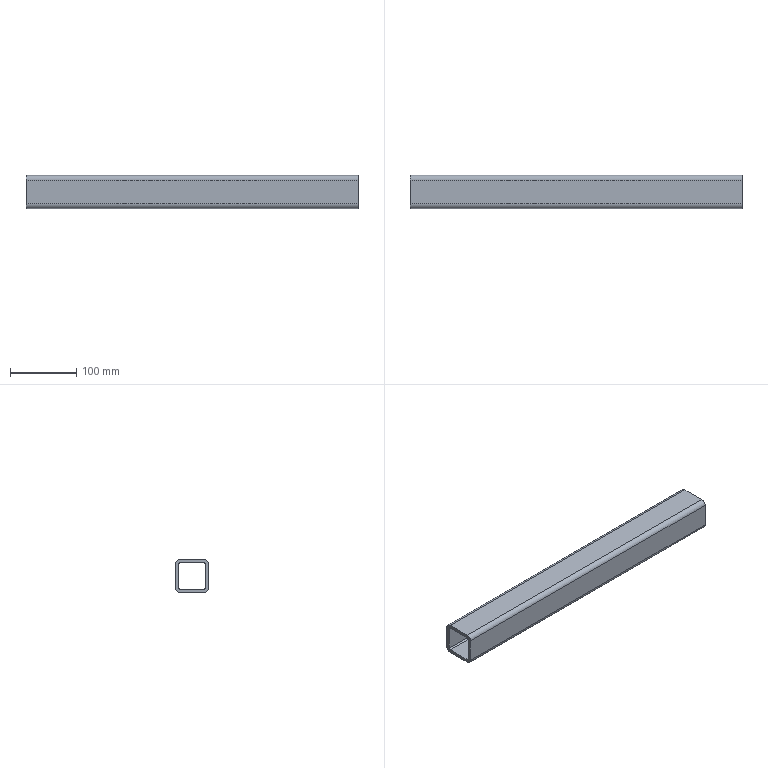Part | NX | 1 solid | 18 faces | box 500 x 50 x 50 mm | volume 430686 mm3 | plane 10 | cylinder 8 | commonest cylinder face diameters 4 x4 14 x4
STEP:
#1=CARTESIAN_POINT('',(-850.,18.,290.));
#2=VERTEX_POINT('',#1);
#3=CARTESIAN_POINT('',(-350.,18.,290.));
#4=VERTEX_POINT('',#3);
#5=CARTESIAN_POINT('',(-875.,18.,290.));
#6=DIRECTION('',(1.,0.,0.));
#7=VECTOR('',#6,1000.);
#8=LINE('',#5,#7);
#9=EDGE_CURVE('',#2,#4,#8,.T.);
#10=ORIENTED_EDGE('',*,*,#9,.F.);
#11=CARTESIAN_POINT('',(-850.,-18.,290.));
#12=VERTEX_POINT('',#11);
#13=CARTESIAN_POINT('',(-850.,-18.,290.));
#14=DIRECTION('',(0.,-1.,0.));
#15=VECTOR('',#14,1000.);
#16=LINE('',#13,#15);
#17=EDGE_CURVE('',#2,#12,#16,.T.);
#18=ORIENTED_EDGE('',*,*,#17,.T.);
#19=CARTESIAN_POINT('',(-350.,-18.,290.));
#20=VERTEX_POINT('',#19);
#21=CARTESIAN_POINT('',(-875.,-18.,290.));
#22=DIRECTION('',(1.,0.,0.));
#23=VECTOR('',#22,1000.);
#24=LINE('',#21,#23);
#25=EDGE_CURVE('',#12,#20,#24,.T.);
#26=ORIENTED_EDGE('',*,*,#25,.T.);
#27=CARTESIAN_POINT('',(-350.,-18.,290.));
#28=DIRECTION('',(0.,1.,0.));
#29=VECTOR('',#28,1000.);
#30=LINE('',#27,#29);
#31=EDGE_CURVE('',#20,#4,#30,.T.);
#32=ORIENTED_EDGE('',*,*,#31,.T.);
#33=EDGE_LOOP('',(#10,#18,#26,#32));
#34=FACE_BOUND('',#33,.T.);
#35=CARTESIAN_POINT('',(-875.,-18.,290.));
#36=DIRECTION('',(0.,0.,1.));
#37=DIRECTION('',(1.,0.,0.));
#38=AXIS2_PLACEMENT_3D('',#35,#36,#37);
#39=PLANE('',#38);
#40=ADVANCED_FACE('',(#34),#39,.T.);
#41=ORIENTED_EDGE('',*,*,#25,.F.);
#42=CARTESIAN_POINT('',(-850.,-20.,292.));
#43=VERTEX_POINT('',#42);
#44=CARTESIAN_POINT('',(-850.,-18.,292.));
#45=DIRECTION('',(-1.,0.,0.));
#46=DIRECTION('',(0.,0.,1.));
#47=AXIS2_PLACEMENT_3D('',#44,#45,#46);
#48=CIRCLE('',#47,2.);
#49=EDGE_CURVE('',#12,#43,#48,.T.);
#50=ORIENTED_EDGE('',*,*,#49,.T.);
#51=CARTESIAN_POINT('',(-350.,-20.,292.));
#52=VERTEX_POINT('',#51);
#53=CARTESIAN_POINT('',(-875.,-20.,292.));
#54=DIRECTION('',(1.,0.,0.));
#55=VECTOR('',#54,1000.);
#56=LINE('',#53,#55);
#57=EDGE_CURVE('',#43,#52,#56,.T.);
#58=ORIENTED_EDGE('',*,*,#57,.T.);
#59=CARTESIAN_POINT('',(-350.,-18.,292.));
#60=DIRECTION('',(1.,0.,0.));
#61=DIRECTION('',(0.,1.,0.));
#62=AXIS2_PLACEMENT_3D('',#59,#60,#61);
#63=CIRCLE('',#62,2.);
#64=EDGE_CURVE('',#52,#20,#63,.T.);
#65=ORIENTED_EDGE('',*,*,#64,.T.);
#66=EDGE_LOOP('',(#41,#50,#58,#65));
#67=FACE_BOUND('',#66,.T.);
#68=CARTESIAN_POINT('',(-875.,-18.,292.));
#69=DIRECTION('',(1.,0.,0.));
#70=DIRECTION('',(0.,0.,-1.));
#71=AXIS2_PLACEMENT_3D('',#68,#69,#70);
#72=CYLINDRICAL_SURFACE('',#71,2.);
#73=ADVANCED_FACE('',(#67),#72,.F.);
#74=ORIENTED_EDGE('',*,*,#57,.F.);
#75=CARTESIAN_POINT('',(-850.,-20.,328.));
#76=VERTEX_POINT('',#75);
#77=CARTESIAN_POINT('',(-850.,-20.,292.));
#78=DIRECTION('',(0.,0.,1.));
#79=VECTOR('',#78,1000.);
#80=LINE('',#77,#79);
#81=EDGE_CURVE('',#43,#76,#80,.T.);
#82=ORIENTED_EDGE('',*,*,#81,.T.);
#83=CARTESIAN_POINT('',(-350.,-20.,328.));
#84=VERTEX_POINT('',#83);
#85=CARTESIAN_POINT('',(-875.,-20.,328.));
#86=DIRECTION('',(1.,0.,0.));
#87=VECTOR('',#86,1000.);
#88=LINE('',#85,#87);
#89=EDGE_CURVE('',#76,#84,#88,.T.);
#90=ORIENTED_EDGE('',*,*,#89,.T.);
#91=CARTESIAN_POINT('',(-350.,-20.,292.));
#92=DIRECTION('',(0.,0.,-1.));
#93=VECTOR('',#92,1000.);
#94=LINE('',#91,#93);
#95=EDGE_CURVE('',#84,#52,#94,.T.);
#96=ORIENTED_EDGE('',*,*,#95,.T.);
#97=EDGE_LOOP('',(#74,#82,#90,#96));
#98=FACE_BOUND('',#97,.T.);
#99=CARTESIAN_POINT('',(-875.,-20.,292.));
#100=DIRECTION('',(0.,1.,0.));
#101=DIRECTION('',(0.,0.,1.));
#102=AXIS2_PLACEMENT_3D('',#99,#100,#101);
#103=PLANE('',#102);
#104=ADVANCED_FACE('',(#98),#103,.T.);
#105=ORIENTED_EDGE('',*,*,#89,.F.);
#106=CARTESIAN_POINT('',(-850.,-18.,330.));
#107=VERTEX_POINT('',#106);
#108=CARTESIAN_POINT('',(-850.,-18.,328.));
#109=DIRECTION('',(-1.,0.,0.));
#110=DIRECTION('',(0.,0.,1.));
#111=AXIS2_PLACEMENT_3D('',#108,#109,#110);
#112=CIRCLE('',#111,2.);
#113=EDGE_CURVE('',#76,#107,#112,.T.);
#114=ORIENTED_EDGE('',*,*,#113,.T.);
#115=CARTESIAN_POINT('',(-350.,-18.,330.));
#116=VERTEX_POINT('',#115);
#117=CARTESIAN_POINT('',(-875.,-18.,330.));
#118=DIRECTION('',(1.,0.,0.));
#119=VECTOR('',#118,1000.);
#120=LINE('',#117,#119);
#121=EDGE_CURVE('',#107,#116,#120,.T.);
#122=ORIENTED_EDGE('',*,*,#121,.T.);
#123=CARTESIAN_POINT('',(-350.,-18.,328.));
#124=DIRECTION('',(1.,0.,0.));
#125=DIRECTION('',(0.,1.,0.));
#126=AXIS2_PLACEMENT_3D('',#123,#124,#125);
#127=CIRCLE('',#126,2.);
#128=EDGE_CURVE('',#116,#84,#127,.T.);
#129=ORIENTED_EDGE('',*,*,#128,.T.);
#130=EDGE_LOOP('',(#105,#114,#122,#129));
#131=FACE_BOUND('',#130,.T.);
#132=CARTESIAN_POINT('',(-875.,-18.,328.));
#133=DIRECTION('',(1.,0.,0.));
#134=DIRECTION('',(0.,0.,-1.));
#135=AXIS2_PLACEMENT_3D('',#132,#133,#134);
#136=CYLINDRICAL_SURFACE('',#135,2.);
#137=ADVANCED_FACE('',(#131),#136,.F.);
#138=ORIENTED_EDGE('',*,*,#121,.F.);
#139=CARTESIAN_POINT('',(-850.,18.,330.));
#140=VERTEX_POINT('',#139);
#141=CARTESIAN_POINT('',(-850.,18.,330.));
#142=DIRECTION('',(0.,1.,0.));
#143=VECTOR('',#142,1000.);
#144=LINE('',#141,#143);
#145=EDGE_CURVE('',#107,#140,#144,.T.);
#146=ORIENTED_EDGE('',*,*,#145,.T.);
#147=CARTESIAN_POINT('',(-350.,18.,330.));
#148=VERTEX_POINT('',#147);
#149=CARTESIAN_POINT('',(-875.,18.,330.));
#150=DIRECTION('',(1.,0.,0.));
#151=VECTOR('',#150,1000.);
#152=LINE('',#149,#151);
#153=EDGE_CURVE('',#140,#148,#152,.T.);
#154=ORIENTED_EDGE('',*,*,#153,.T.);
#155=CARTESIAN_POINT('',(-350.,18.,330.));
#156=DIRECTION('',(0.,-1.,0.));
#157=VECTOR('',#156,1000.);
#158=LINE('',#155,#157);
#159=EDGE_CURVE('',#148,#116,#158,.T.);
#160=ORIENTED_EDGE('',*,*,#159,.T.);
#161=EDGE_LOOP('',(#138,#146,#154,#160));
#162=FACE_BOUND('',#161,.T.);
#163=CARTESIAN_POINT('',(-875.,18.,330.));
#164=DIRECTION('',(0.,0.,-1.));
#165=DIRECTION('',(-1.,0.,0.));
#166=AXIS2_PLACEMENT_3D('',#163,#164,#165);
#167=PLANE('',#166);
#168=ADVANCED_FACE('',(#162),#167,.T.);
#169=ORIENTED_EDGE('',*,*,#153,.F.);
#170=CARTESIAN_POINT('',(-850.,20.,328.));
#171=VERTEX_POINT('',#170);
#172=CARTESIAN_POINT('',(-850.,18.,328.));
#173=DIRECTION('',(-1.,0.,0.));
#174=DIRECTION('',(0.,0.,1.));
#175=AXIS2_PLACEMENT_3D('',#172,#173,#174);
#176=CIRCLE('',#175,2.);
#177=EDGE_CURVE('',#140,#171,#176,.T.);
#178=ORIENTED_EDGE('',*,*,#177,.T.);
#179=CARTESIAN_POINT('',(-350.,20.,328.));
#180=VERTEX_POINT('',#179);
#181=CARTESIAN_POINT('',(-875.,20.,328.));
#182=DIRECTION('',(1.,0.,0.));
#183=VECTOR('',#182,1000.);
#184=LINE('',#181,#183);
#185=EDGE_CURVE('',#171,#180,#184,.T.);
#186=ORIENTED_EDGE('',*,*,#185,.T.);
#187=CARTESIAN_POINT('',(-350.,18.,328.));
#188=DIRECTION('',(1.,0.,0.));
#189=DIRECTION('',(0.,1.,0.));
#190=AXIS2_PLACEMENT_3D('',#187,#188,#189);
#191=CIRCLE('',#190,2.);
#192=EDGE_CURVE('',#180,#148,#191,.T.);
#193=ORIENTED_EDGE('',*,*,#192,.T.);
#194=EDGE_LOOP('',(#169,#178,#186,#193));
#195=FACE_BOUND('',#194,.T.);
#196=CARTESIAN_POINT('',(-875.,18.,328.));
#197=DIRECTION('',(1.,0.,0.));
#198=DIRECTION('',(0.,0.,-1.));
#199=AXIS2_PLACEMENT_3D('',#196,#197,#198);
#200=CYLINDRICAL_SURFACE('',#199,2.);
#201=ADVANCED_FACE('',(#195),#200,.F.);
#202=ORIENTED_EDGE('',*,*,#185,.F.);
#203=CARTESIAN_POINT('',(-850.,20.,292.));
#204=VERTEX_POINT('',#203);
#205=CARTESIAN_POINT('',(-850.,20.,328.));
#206=DIRECTION('',(0.,0.,-1.));
#207=VECTOR('',#206,1000.);
#208=LINE('',#205,#207);
#209=EDGE_CURVE('',#171,#204,#208,.T.);
#210=ORIENTED_EDGE('',*,*,#209,.T.);
#211=CARTESIAN_POINT('',(-350.,20.,292.));
#212=VERTEX_POINT('',#211);
#213=CARTESIAN_POINT('',(-875.,20.,292.));
#214=DIRECTION('',(1.,0.,0.));
#215=VECTOR('',#214,1000.);
#216=LINE('',#213,#215);
#217=EDGE_CURVE('',#204,#212,#216,.T.);
#218=ORIENTED_EDGE('',*,*,#217,.T.);
#219=CARTESIAN_POINT('',(-350.,20.,328.));
#220=DIRECTION('',(0.,0.,1.));
#221=VECTOR('',#220,1000.);
#222=LINE('',#219,#221);
#223=EDGE_CURVE('',#212,#180,#222,.T.);
#224=ORIENTED_EDGE('',*,*,#223,.T.);
#225=EDGE_LOOP('',(#202,#210,#218,#224));
#226=FACE_BOUND('',#225,.T.);
#227=CARTESIAN_POINT('',(-875.,20.,328.));
#228=DIRECTION('',(0.,-1.,0.));
#229=DIRECTION('',(0.,0.,-1.));
#230=AXIS2_PLACEMENT_3D('',#227,#228,#229);
#231=PLANE('',#230);
#232=ADVANCED_FACE('',(#226),#231,.T.);
#233=ORIENTED_EDGE('',*,*,#217,.F.);
#234=CARTESIAN_POINT('',(-850.,18.,292.));
#235=DIRECTION('',(-1.,0.,0.));
#236=DIRECTION('',(0.,0.,1.));
#237=AXIS2_PLACEMENT_3D('',#234,#235,#236);
#238=CIRCLE('',#237,2.);
#239=EDGE_CURVE('',#204,#2,#238,.T.);
#240=ORIENTED_EDGE('',*,*,#239,.T.);
#241=ORIENTED_EDGE('',*,*,#9,.T.);
#242=CARTESIAN_POINT('',(-350.,18.,292.));
#243=DIRECTION('',(1.,0.,0.));
#244=DIRECTION('',(0.,1.,0.));
#245=AXIS2_PLACEMENT_3D('',#242,#243,#244);
#246=CIRCLE('',#245,2.);
#247=EDGE_CURVE('',#4,#212,#246,.T.);
#248=ORIENTED_EDGE('',*,*,#247,.T.);
#249=EDGE_LOOP('',(#233,#240,#241,#248));
#250=FACE_BOUND('',#249,.T.);
#251=CARTESIAN_POINT('',(-875.,18.,292.));
#252=DIRECTION('',(1.,0.,0.));
#253=DIRECTION('',(0.,0.,-1.));
#254=AXIS2_PLACEMENT_3D('',#251,#252,#253);
#255=CYLINDRICAL_SURFACE('',#254,2.);
#256=ADVANCED_FACE('',(#250),#255,.F.);
#257=CARTESIAN_POINT('',(-850.,-18.,335.));
#258=VERTEX_POINT('',#257);
#259=CARTESIAN_POINT('',(-850.,18.,335.));
#260=VERTEX_POINT('',#259);
#261=CARTESIAN_POINT('',(-850.,0.,335.));
#262=DIRECTION('',(0.,1.,0.));
#263=VECTOR('',#262,1000.);
#264=LINE('',#261,#263);
#265=EDGE_CURVE('',#258,#260,#264,.T.);
#266=ORIENTED_EDGE('',*,*,#265,.F.);
#267=CARTESIAN_POINT('',(-350.,-18.,335.));
#268=VERTEX_POINT('',#267);
#269=CARTESIAN_POINT('',(-875.,-18.,335.));
#270=DIRECTION('',(1.,0.,0.));
#271=VECTOR('',#270,1000.);
#272=LINE('',#269,#271);
#273=EDGE_CURVE('',#258,#268,#272,.T.);
#274=ORIENTED_EDGE('',*,*,#273,.T.);
#275=CARTESIAN_POINT('',(-350.,18.,335.));
#276=VERTEX_POINT('',#275);
#277=CARTESIAN_POINT('',(-350.,18.,335.));
#278=DIRECTION('',(0.,-1.,0.));
#279=VECTOR('',#278,1000.);
#280=LINE('',#277,#279);
#281=EDGE_CURVE('',#276,#268,#280,.T.);
#282=ORIENTED_EDGE('',*,*,#281,.F.);
#283=CARTESIAN_POINT('',(-875.,18.,335.));
#284=DIRECTION('',(1.,0.,0.));
#285=VECTOR('',#284,1000.);
#286=LINE('',#283,#285);
#287=EDGE_CURVE('',#260,#276,#286,.T.);
#288=ORIENTED_EDGE('',*,*,#287,.F.);
#289=EDGE_LOOP('',(#266,#274,#282,#288));
#290=FACE_BOUND('',#289,.T.);
#291=CARTESIAN_POINT('',(-875.,18.,335.));
#292=DIRECTION('',(0.,0.,-1.));
#293=DIRECTION('',(-1.,0.,0.));
#294=AXIS2_PLACEMENT_3D('',#291,#292,#293);
#295=PLANE('',#294);
#296=ADVANCED_FACE('',(#290),#295,.F.);
#297=CARTESIAN_POINT('',(-850.,-25.,328.));
#298=VERTEX_POINT('',#297);
#299=CARTESIAN_POINT('',(-850.,-18.,328.));
#300=DIRECTION('',(-1.,0.,0.));
#301=DIRECTION('',(0.,0.,1.));
#302=AXIS2_PLACEMENT_3D('',#299,#300,#301);
#303=CIRCLE('',#302,7.);
#304=EDGE_CURVE('',#298,#258,#303,.T.);
#305=ORIENTED_EDGE('',*,*,#304,.F.);
#306=CARTESIAN_POINT('',(-350.,-25.,328.));
#307=VERTEX_POINT('',#306);
#308=CARTESIAN_POINT('',(-875.,-25.,328.));
#309=DIRECTION('',(1.,0.,0.));
#310=VECTOR('',#309,1000.);
#311=LINE('',#308,#310);
#312=EDGE_CURVE('',#298,#307,#311,.T.);
#313=ORIENTED_EDGE('',*,*,#312,.T.);
#314=CARTESIAN_POINT('',(-350.,-18.,328.));
#315=DIRECTION('',(1.,0.,0.));
#316=DIRECTION('',(0.,1.,0.));
#317=AXIS2_PLACEMENT_3D('',#314,#315,#316);
#318=CIRCLE('',#317,7.);
#319=EDGE_CURVE('',#268,#307,#318,.T.);
#320=ORIENTED_EDGE('',*,*,#319,.F.);
#321=ORIENTED_EDGE('',*,*,#273,.F.);
#322=EDGE_LOOP('',(#305,#313,#320,#321));
#323=FACE_BOUND('',#322,.T.);
#324=CARTESIAN_POINT('',(-875.,-18.,328.));
#325=DIRECTION('',(1.,0.,0.));
#326=DIRECTION('',(0.,0.,-1.));
#327=AXIS2_PLACEMENT_3D('',#324,#325,#326);
#328=CYLINDRICAL_SURFACE('',#327,7.);
#329=ADVANCED_FACE('',(#323),#328,.T.);
#330=CARTESIAN_POINT('',(-850.,-25.,292.));
#331=VERTEX_POINT('',#330);
#332=CARTESIAN_POINT('',(-850.,-25.,292.));
#333=DIRECTION('',(0.,0.,1.));
#334=VECTOR('',#333,1000.);
#335=LINE('',#332,#334);
#336=EDGE_CURVE('',#331,#298,#335,.T.);
#337=ORIENTED_EDGE('',*,*,#336,.F.);
#338=CARTESIAN_POINT('',(-350.,-25.,292.));
#339=VERTEX_POINT('',#338);
#340=CARTESIAN_POINT('',(-875.,-25.,292.));
#341=DIRECTION('',(1.,0.,0.));
#342=VECTOR('',#341,1000.);
#343=LINE('',#340,#342);
#344=EDGE_CURVE('',#331,#339,#343,.T.);
#345=ORIENTED_EDGE('',*,*,#344,.T.);
#346=CARTESIAN_POINT('',(-350.,-25.,575.));
#347=DIRECTION('',(0.,0.,-1.));
#348=VECTOR('',#347,1000.);
#349=LINE('',#346,#348);
#350=EDGE_CURVE('',#307,#339,#349,.T.);
#351=ORIENTED_EDGE('',*,*,#350,.F.);
#352=ORIENTED_EDGE('',*,*,#312,.F.);
#353=EDGE_LOOP('',(#337,#345,#351,#352));
#354=FACE_BOUND('',#353,.T.);
#355=CARTESIAN_POINT('',(-875.,-25.,292.));
#356=DIRECTION('',(0.,1.,0.));
#357=DIRECTION('',(0.,0.,1.));
#358=AXIS2_PLACEMENT_3D('',#355,#356,#357);
#359=PLANE('',#358);
#360=ADVANCED_FACE('',(#354),#359,.F.);
#361=CARTESIAN_POINT('',(-850.,-18.,285.));
#362=VERTEX_POINT('',#361);
#363=CARTESIAN_POINT('',(-850.,-18.,292.));
#364=DIRECTION('',(-1.,0.,0.));
#365=DIRECTION('',(0.,0.,1.));
#366=AXIS2_PLACEMENT_3D('',#363,#364,#365);
#367=CIRCLE('',#366,7.);
#368=EDGE_CURVE('',#362,#331,#367,.T.);
#369=ORIENTED_EDGE('',*,*,#368,.F.);
#370=CARTESIAN_POINT('',(-350.,-18.,285.));
#371=VERTEX_POINT('',#370);
#372=CARTESIAN_POINT('',(-875.,-18.,285.));
#373=DIRECTION('',(1.,0.,0.));
#374=VECTOR('',#373,1000.);
#375=LINE('',#372,#374);
#376=EDGE_CURVE('',#362,#371,#375,.T.);
#377=ORIENTED_EDGE('',*,*,#376,.T.);
#378=CARTESIAN_POINT('',(-350.,-18.,292.));
#379=DIRECTION('',(1.,0.,0.));
#380=DIRECTION('',(0.,1.,0.));
#381=AXIS2_PLACEMENT_3D('',#378,#379,#380);
#382=CIRCLE('',#381,7.);
#383=EDGE_CURVE('',#339,#371,#382,.T.);
#384=ORIENTED_EDGE('',*,*,#383,.F.);
#385=ORIENTED_EDGE('',*,*,#344,.F.);
#386=EDGE_LOOP('',(#369,#377,#384,#385));
#387=FACE_BOUND('',#386,.T.);
#388=CARTESIAN_POINT('',(-875.,-18.,292.));
#389=DIRECTION('',(1.,0.,0.));
#390=DIRECTION('',(0.,0.,-1.));
#391=AXIS2_PLACEMENT_3D('',#388,#389,#390);
#392=CYLINDRICAL_SURFACE('',#391,7.);
#393=ADVANCED_FACE('',(#387),#392,.T.);
#394=CARTESIAN_POINT('',(-850.,18.,285.));
#395=VERTEX_POINT('',#394);
#396=CARTESIAN_POINT('',(-850.,0.,285.));
#397=DIRECTION('',(0.,1.,0.));
#398=VECTOR('',#397,1000.);
#399=LINE('',#396,#398);
#400=EDGE_CURVE('',#362,#395,#399,.T.);
#401=ORIENTED_EDGE('',*,*,#400,.T.);
#402=CARTESIAN_POINT('',(-350.,18.,285.));
#403=VERTEX_POINT('',#402);
#404=CARTESIAN_POINT('',(-875.,18.,285.));
#405=DIRECTION('',(1.,0.,0.));
#406=VECTOR('',#405,1000.);
#407=LINE('',#404,#406);
#408=EDGE_CURVE('',#395,#403,#407,.T.);
#409=ORIENTED_EDGE('',*,*,#408,.T.);
#410=CARTESIAN_POINT('',(-350.,-18.,285.));
#411=DIRECTION('',(0.,1.,0.));
#412=VECTOR('',#411,1000.);
#413=LINE('',#410,#412);
#414=EDGE_CURVE('',#371,#403,#413,.T.);
#415=ORIENTED_EDGE('',*,*,#414,.F.);
#416=ORIENTED_EDGE('',*,*,#376,.F.);
#417=EDGE_LOOP('',(#401,#409,#415,#416));
#418=FACE_BOUND('',#417,.T.);
#419=CARTESIAN_POINT('',(-875.,-18.,285.));
#420=DIRECTION('',(0.,0.,1.));
#421=DIRECTION('',(1.,0.,0.));
#422=AXIS2_PLACEMENT_3D('',#419,#420,#421);
#423=PLANE('',#422);
#424=ADVANCED_FACE('',(#418),#423,.F.);
#425=CARTESIAN_POINT('',(-850.,25.,292.));
#426=VERTEX_POINT('',#425);
#427=CARTESIAN_POINT('',(-850.,18.,292.));
#428=DIRECTION('',(-1.,0.,0.));
#429=DIRECTION('',(0.,0.,1.));
#430=AXIS2_PLACEMENT_3D('',#427,#428,#429);
#431=CIRCLE('',#430,7.);
#432=EDGE_CURVE('',#426,#395,#431,.T.);
#433=ORIENTED_EDGE('',*,*,#432,.F.);
#434=CARTESIAN_POINT('',(-350.,25.,292.));
#435=VERTEX_POINT('',#434);
#436=CARTESIAN_POINT('',(-875.,25.,292.));
#437=DIRECTION('',(1.,0.,0.));
#438=VECTOR('',#437,1000.);
#439=LINE('',#436,#438);
#440=EDGE_CURVE('',#426,#435,#439,.T.);
#441=ORIENTED_EDGE('',*,*,#440,.T.);
#442=CARTESIAN_POINT('',(-350.,18.,292.));
#443=DIRECTION('',(1.,0.,0.));
#444=DIRECTION('',(0.,1.,0.));
#445=AXIS2_PLACEMENT_3D('',#442,#443,#444);
#446=CIRCLE('',#445,7.);
#447=EDGE_CURVE('',#403,#435,#446,.T.);
#448=ORIENTED_EDGE('',*,*,#447,.F.);
#449=ORIENTED_EDGE('',*,*,#408,.F.);
#450=EDGE_LOOP('',(#433,#441,#448,#449));
#451=FACE_BOUND('',#450,.T.);
#452=CARTESIAN_POINT('',(-875.,18.,292.));
#453=DIRECTION('',(1.,0.,0.));
#454=DIRECTION('',(0.,0.,-1.));
#455=AXIS2_PLACEMENT_3D('',#452,#453,#454);
#456=CYLINDRICAL_SURFACE('',#455,7.);
#457=ADVANCED_FACE('',(#451),#456,.T.);
#458=CARTESIAN_POINT('',(-850.,25.,328.));
#459=VERTEX_POINT('',#458);
#460=CARTESIAN_POINT('',(-850.,25.,328.));
#461=DIRECTION('',(0.,0.,-1.));
#462=VECTOR('',#461,1000.);
#463=LINE('',#460,#462);
#464=EDGE_CURVE('',#459,#426,#463,.T.);
#465=ORIENTED_EDGE('',*,*,#464,.F.);
#466=CARTESIAN_POINT('',(-350.,25.,328.));
#467=VERTEX_POINT('',#466);
#468=CARTESIAN_POINT('',(-875.,25.,328.));
#469=DIRECTION('',(1.,0.,0.));
#470=VECTOR('',#469,1000.);
#471=LINE('',#468,#470);
#472=EDGE_CURVE('',#459,#467,#471,.T.);
#473=ORIENTED_EDGE('',*,*,#472,.T.);
#474=CARTESIAN_POINT('',(-350.,25.,575.));
#475=DIRECTION('',(0.,0.,-1.));
#476=VECTOR('',#475,1000.);
#477=LINE('',#474,#476);
#478=EDGE_CURVE('',#467,#435,#477,.T.);
#479=ORIENTED_EDGE('',*,*,#478,.T.);
#480=ORIENTED_EDGE('',*,*,#440,.F.);
#481=EDGE_LOOP('',(#465,#473,#479,#480));
#482=FACE_BOUND('',#481,.T.);
#483=CARTESIAN_POINT('',(-875.,25.,328.));
#484=DIRECTION('',(0.,-1.,0.));
#485=DIRECTION('',(0.,0.,-1.));
#486=AXIS2_PLACEMENT_3D('',#483,#484,#485);
#487=PLANE('',#486);
#488=ADVANCED_FACE('',(#482),#487,.F.);
#489=CARTESIAN_POINT('',(-850.,18.,328.));
#490=DIRECTION('',(-1.,0.,0.));
#491=DIRECTION('',(0.,0.,1.));
#492=AXIS2_PLACEMENT_3D('',#489,#490,#491);
#493=CIRCLE('',#492,7.);
#494=EDGE_CURVE('',#260,#459,#493,.T.);
#495=ORIENTED_EDGE('',*,*,#494,.F.);
#496=ORIENTED_EDGE('',*,*,#287,.T.);
#497=CARTESIAN_POINT('',(-350.,18.,328.));
#498=DIRECTION('',(1.,0.,0.));
#499=DIRECTION('',(0.,1.,0.));
#500=AXIS2_PLACEMENT_3D('',#497,#498,#499);
#501=CIRCLE('',#500,7.);
#502=EDGE_CURVE('',#467,#276,#501,.T.);
#503=ORIENTED_EDGE('',*,*,#502,.F.);
#504=ORIENTED_EDGE('',*,*,#472,.F.);
#505=EDGE_LOOP('',(#495,#496,#503,#504));
#506=FACE_BOUND('',#505,.T.);
#507=CARTESIAN_POINT('',(-875.,18.,328.));
#508=DIRECTION('',(1.,0.,0.));
#509=DIRECTION('',(0.,0.,-1.));
#510=AXIS2_PLACEMENT_3D('',#507,#508,#509);
#511=CYLINDRICAL_SURFACE('',#510,7.);
#512=ADVANCED_FACE('',(#506),#511,.T.);
#513=ORIENTED_EDGE('',*,*,#31,.F.);
#514=ORIENTED_EDGE('',*,*,#64,.F.);
#515=ORIENTED_EDGE('',*,*,#95,.F.);
#516=ORIENTED_EDGE('',*,*,#128,.F.);
#517=ORIENTED_EDGE('',*,*,#159,.F.);
#518=ORIENTED_EDGE('',*,*,#192,.F.);
#519=ORIENTED_EDGE('',*,*,#223,.F.);
#520=ORIENTED_EDGE('',*,*,#247,.F.);
#521=EDGE_LOOP('',(#513,#514,#515,#516,#517,#518,#519,#520));
#522=FACE_BOUND('',#521,.T.);
#523=ORIENTED_EDGE('',*,*,#447,.T.);
#524=ORIENTED_EDGE('',*,*,#478,.F.);
#525=ORIENTED_EDGE('',*,*,#502,.T.);
#526=ORIENTED_EDGE('',*,*,#281,.T.);
#527=ORIENTED_EDGE('',*,*,#319,.T.);
#528=ORIENTED_EDGE('',*,*,#350,.T.);
#529=ORIENTED_EDGE('',*,*,#383,.T.);
#530=ORIENTED_EDGE('',*,*,#414,.T.);
#531=EDGE_LOOP('',(#523,#524,#525,#526,#527,#528,#529,#530));
#532=FACE_BOUND('',#531,.T.);
#533=CARTESIAN_POINT('',(-350.,-18.,575.));
#534=DIRECTION('',(1.,0.,0.));
#535=DIRECTION('',(0.,1.,0.));
#536=AXIS2_PLACEMENT_3D('',#533,#534,#535);
#537=PLANE('',#536);
#538=ADVANCED_FACE('',(#522,#532),#537,.T.);
#539=ORIENTED_EDGE('',*,*,#239,.F.);
#540=ORIENTED_EDGE('',*,*,#209,.F.);
#541=ORIENTED_EDGE('',*,*,#177,.F.);
#542=ORIENTED_EDGE('',*,*,#145,.F.);
#543=ORIENTED_EDGE('',*,*,#113,.F.);
#544=ORIENTED_EDGE('',*,*,#81,.F.);
#545=ORIENTED_EDGE('',*,*,#49,.F.);
#546=ORIENTED_EDGE('',*,*,#17,.F.);
#547=EDGE_LOOP('',(#539,#540,#541,#542,#543,#544,#545,#546));
#548=FACE_BOUND('',#547,.T.);
#549=ORIENTED_EDGE('',*,*,#304,.T.);
#550=ORIENTED_EDGE('',*,*,#265,.T.);
#551=ORIENTED_EDGE('',*,*,#494,.T.);
#552=ORIENTED_EDGE('',*,*,#464,.T.);
#553=ORIENTED_EDGE('',*,*,#432,.T.);
#554=ORIENTED_EDGE('',*,*,#400,.F.);
#555=ORIENTED_EDGE('',*,*,#368,.T.);
#556=ORIENTED_EDGE('',*,*,#336,.T.);
#557=EDGE_LOOP('',(#549,#550,#551,#552,#553,#554,#555,#556));
#558=FACE_BOUND('',#557,.T.);
#559=CARTESIAN_POINT('',(-850.,0.,328.));
#560=DIRECTION('',(-1.,0.,0.));
#561=DIRECTION('',(0.,0.,1.));
#562=AXIS2_PLACEMENT_3D('',#559,#560,#561);
#563=PLANE('',#562);
#564=ADVANCED_FACE('',(#548,#558),#563,.T.);
#565=CLOSED_SHELL('',(#40,#73,#104,#137,#168,#201,#232,#256,#296,#329,#360,#393,#424,#457,#488,#512,#538,#564));
#566=MANIFOLD_SOLID_BREP('',#565);
#567=(LENGTH_UNIT()NAMED_UNIT(*)SI_UNIT(.MILLI.,.METRE.));
#568=UNCERTAINTY_MEASURE_WITH_UNIT(LENGTH_MEASURE(0.00001),#567,'','');
#569=(NAMED_UNIT(*)PLANE_ANGLE_UNIT()SI_UNIT($,.RADIAN.));
#570=(NAMED_UNIT(*)SI_UNIT($,.STERADIAN.)SOLID_ANGLE_UNIT());
#571=(GEOMETRIC_REPRESENTATION_CONTEXT(3)GLOBAL_UNCERTAINTY_ASSIGNED_CONTEXT((#568))GLOBAL_UNIT_ASSIGNED_CONTEXT((#567,#569,#570))REPRESENTATION_CONTEXT('',''));
#572=ADVANCED_BREP_SHAPE_REPRESENTATION('',(#566),#571);